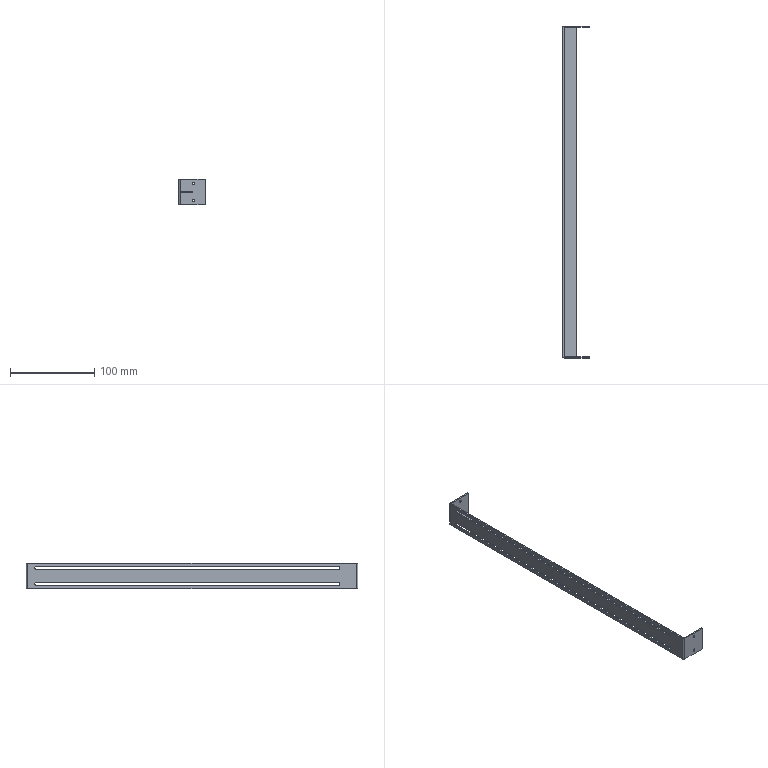Part | SolidWorks | features ICE 3, FlatPattern 1, SMBaseFlange 1, SheetMetal 1 | 1 solid | 46 faces | box 31.5 x 395 x 30 mm | volume 22778 mm3 | plane 26 | cylinder 20 | commonest cylinder face diameters 3.2 x14 1 x4 4 x2
STEP:
#1=CARTESIAN_POINT('',(0.,-174.5,26.2));
#2=VERTEX_POINT('',#1);
#3=CARTESIAN_POINT('',(0.,-176.1,24.6));
#4=VERTEX_POINT('',#3);
#5=CARTESIAN_POINT('',(0.,-174.5,24.6));
#6=DIRECTION('',(1.,0.,0.));
#7=DIRECTION('',(0.,1.,0.));
#8=AXIS2_PLACEMENT_3D('',#5,#6,#7);
#9=CIRCLE('',#8,1.6);
#10=EDGE_CURVE('',#2,#4,#9,.T.);
#11=ORIENTED_EDGE('',*,*,#10,.T.);
#12=CARTESIAN_POINT('',(-1.5,-176.1,24.6));
#13=VERTEX_POINT('',#12);
#14=CARTESIAN_POINT('',(30.,-176.1,24.6));
#15=DIRECTION('',(-1.,0.,0.));
#16=VECTOR('',#15,1000.);
#17=LINE('',#14,#16);
#18=EDGE_CURVE('',#4,#13,#17,.T.);
#19=ORIENTED_EDGE('',*,*,#18,.T.);
#20=CARTESIAN_POINT('',(-1.5,-174.5,26.2));
#21=VERTEX_POINT('',#20);
#22=CARTESIAN_POINT('',(-1.5,-174.5,24.6));
#23=DIRECTION('',(-1.,0.,0.));
#24=DIRECTION('',(0.,-1.,0.));
#25=AXIS2_PLACEMENT_3D('',#22,#23,#24);
#26=CIRCLE('',#25,1.6);
#27=EDGE_CURVE('',#13,#21,#26,.T.);
#28=ORIENTED_EDGE('',*,*,#27,.T.);
#29=CARTESIAN_POINT('',(30.,-174.5,26.2));
#30=DIRECTION('',(-1.,0.,0.));
#31=VECTOR('',#30,1000.);
#32=LINE('',#29,#31);
#33=EDGE_CURVE('',#2,#21,#32,.T.);
#34=ORIENTED_EDGE('',*,*,#33,.F.);
#35=EDGE_LOOP('',(#11,#19,#28,#34));
#36=FACE_OUTER_BOUND('',#35,.T.);
#37=CARTESIAN_POINT('',(30.,-174.5,24.6));
#38=DIRECTION('',(-1.,0.,0.));
#39=DIRECTION('',(0.,-1.,0.));
#40=AXIS2_PLACEMENT_3D('',#37,#38,#39);
#41=CYLINDRICAL_SURFACE('',#40,1.6);
#42=ADVANCED_FACE('',(#36),#41,.F.);
#43=CARTESIAN_POINT('',(0.,-174.5,7.2));
#44=VERTEX_POINT('',#43);
#45=CARTESIAN_POINT('',(0.,-176.1,5.6));
#46=VERTEX_POINT('',#45);
#47=CARTESIAN_POINT('',(0.,-174.5,5.6));
#48=DIRECTION('',(1.,0.,0.));
#49=DIRECTION('',(0.,1.,0.));
#50=AXIS2_PLACEMENT_3D('',#47,#48,#49);
#51=CIRCLE('',#50,1.6);
#52=EDGE_CURVE('',#44,#46,#51,.T.);
#53=ORIENTED_EDGE('',*,*,#52,.T.);
#54=CARTESIAN_POINT('',(-1.5,-176.1,5.6));
#55=VERTEX_POINT('',#54);
#56=CARTESIAN_POINT('',(30.,-176.1,5.6));
#57=DIRECTION('',(-1.,0.,0.));
#58=VECTOR('',#57,1000.);
#59=LINE('',#56,#58);
#60=EDGE_CURVE('',#46,#55,#59,.T.);
#61=ORIENTED_EDGE('',*,*,#60,.T.);
#62=CARTESIAN_POINT('',(-1.5,-174.5,7.2));
#63=VERTEX_POINT('',#62);
#64=CARTESIAN_POINT('',(-1.5,-174.5,5.6));
#65=DIRECTION('',(-1.,0.,0.));
#66=DIRECTION('',(0.,-1.,0.));
#67=AXIS2_PLACEMENT_3D('',#64,#65,#66);
#68=CIRCLE('',#67,1.6);
#69=EDGE_CURVE('',#55,#63,#68,.T.);
#70=ORIENTED_EDGE('',*,*,#69,.T.);
#71=CARTESIAN_POINT('',(30.,-174.5,7.2));
#72=DIRECTION('',(-1.,0.,0.));
#73=VECTOR('',#72,1000.);
#74=LINE('',#71,#73);
#75=EDGE_CURVE('',#44,#63,#74,.T.);
#76=ORIENTED_EDGE('',*,*,#75,.F.);
#77=EDGE_LOOP('',(#53,#61,#70,#76));
#78=FACE_OUTER_BOUND('',#77,.T.);
#79=CARTESIAN_POINT('',(30.,-174.5,5.6));
#80=DIRECTION('',(-1.,0.,0.));
#81=DIRECTION('',(0.,-1.,0.));
#82=AXIS2_PLACEMENT_3D('',#79,#80,#81);
#83=CYLINDRICAL_SURFACE('',#82,1.6);
#84=ADVANCED_FACE('',(#78),#83,.F.);
#85=CARTESIAN_POINT('',(16.,-196.,3.4));
#86=VERTEX_POINT('',#85);
#87=CARTESIAN_POINT('',(16.,-196.,6.6));
#88=VERTEX_POINT('',#87);
#89=CARTESIAN_POINT('',(16.,-196.,5.));
#90=DIRECTION('',(0.,1.,0.));
#91=DIRECTION('',(0.,0.,1.));
#92=AXIS2_PLACEMENT_3D('',#89,#90,#91);
#93=CIRCLE('',#92,1.6);
#94=EDGE_CURVE('',#86,#88,#93,.T.);
#95=ORIENTED_EDGE('',*,*,#94,.T.);
#96=CARTESIAN_POINT('',(16.,-197.5,6.6));
#97=VERTEX_POINT('',#96);
#98=CARTESIAN_POINT('',(16.,197.5,6.6));
#99=DIRECTION('',(0.,-1.,0.));
#100=VECTOR('',#99,1000.);
#101=LINE('',#98,#100);
#102=EDGE_CURVE('',#88,#97,#101,.T.);
#103=ORIENTED_EDGE('',*,*,#102,.T.);
#104=CARTESIAN_POINT('',(16.,-197.5,3.4));
#105=VERTEX_POINT('',#104);
#106=CARTESIAN_POINT('',(16.,-197.5,5.));
#107=DIRECTION('',(0.,-1.,0.));
#108=DIRECTION('',(0.,0.,-1.));
#109=AXIS2_PLACEMENT_3D('',#106,#107,#108);
#110=CIRCLE('',#109,1.6);
#111=EDGE_CURVE('',#97,#105,#110,.T.);
#112=ORIENTED_EDGE('',*,*,#111,.T.);
#113=CARTESIAN_POINT('',(16.,197.5,3.4));
#114=DIRECTION('',(0.,-1.,0.));
#115=VECTOR('',#114,1000.);
#116=LINE('',#113,#115);
#117=EDGE_CURVE('',#86,#105,#116,.T.);
#118=ORIENTED_EDGE('',*,*,#117,.F.);
#119=EDGE_LOOP('',(#95,#103,#112,#118));
#120=FACE_OUTER_BOUND('',#119,.T.);
#121=CARTESIAN_POINT('',(16.,197.5,5.));
#122=DIRECTION('',(0.,-1.,0.));
#123=DIRECTION('',(0.,0.,-1.));
#124=AXIS2_PLACEMENT_3D('',#121,#122,#123);
#125=CYLINDRICAL_SURFACE('',#124,1.6);
#126=ADVANCED_FACE('',(#120),#125,.F.);
#127=CARTESIAN_POINT('',(16.,197.5,6.6));
#128=VERTEX_POINT('',#127);
#129=CARTESIAN_POINT('',(16.,197.5,3.4));
#130=VERTEX_POINT('',#129);
#131=CARTESIAN_POINT('',(16.,197.5,5.));
#132=DIRECTION('',(0.,-1.,0.));
#133=DIRECTION('',(0.,0.,-1.));
#134=AXIS2_PLACEMENT_3D('',#131,#132,#133);
#135=CIRCLE('',#134,1.6);
#136=EDGE_CURVE('',#128,#130,#135,.T.);
#137=ORIENTED_EDGE('',*,*,#136,.F.);
#138=CARTESIAN_POINT('',(16.,196.,6.6));
#139=VERTEX_POINT('',#138);
#140=CARTESIAN_POINT('',(16.,197.5,6.6));
#141=DIRECTION('',(0.,-1.,0.));
#142=VECTOR('',#141,1000.);
#143=LINE('',#140,#142);
#144=EDGE_CURVE('',#128,#139,#143,.T.);
#145=ORIENTED_EDGE('',*,*,#144,.T.);
#146=CARTESIAN_POINT('',(16.,196.,3.4));
#147=VERTEX_POINT('',#146);
#148=CARTESIAN_POINT('',(16.,196.,5.));
#149=DIRECTION('',(0.,-1.,0.));
#150=DIRECTION('',(0.,0.,-1.));
#151=AXIS2_PLACEMENT_3D('',#148,#149,#150);
#152=CIRCLE('',#151,1.6);
#153=EDGE_CURVE('',#139,#147,#152,.T.);
#154=ORIENTED_EDGE('',*,*,#153,.T.);
#155=CARTESIAN_POINT('',(16.,197.5,3.4));
#156=DIRECTION('',(0.,-1.,0.));
#157=VECTOR('',#156,1000.);
#158=LINE('',#155,#157);
#159=EDGE_CURVE('',#130,#147,#158,.T.);
#160=ORIENTED_EDGE('',*,*,#159,.F.);
#161=EDGE_LOOP('',(#137,#145,#154,#160));
#162=FACE_OUTER_BOUND('',#161,.T.);
#163=CARTESIAN_POINT('',(16.,197.5,5.));
#164=DIRECTION('',(0.,-1.,0.));
#165=DIRECTION('',(0.,0.,-1.));
#166=AXIS2_PLACEMENT_3D('',#163,#164,#165);
#167=CYLINDRICAL_SURFACE('',#166,1.6);
#168=ADVANCED_FACE('',(#162),#167,.F.);
#169=CARTESIAN_POINT('',(16.,-196.,23.4));
#170=VERTEX_POINT('',#169);
#171=CARTESIAN_POINT('',(16.,-196.,26.6));
#172=VERTEX_POINT('',#171);
#173=CARTESIAN_POINT('',(16.,-196.,25.));
#174=DIRECTION('',(0.,1.,0.));
#175=DIRECTION('',(0.,0.,1.));
#176=AXIS2_PLACEMENT_3D('',#173,#174,#175);
#177=CIRCLE('',#176,1.6);
#178=EDGE_CURVE('',#170,#172,#177,.T.);
#179=ORIENTED_EDGE('',*,*,#178,.T.);
#180=CARTESIAN_POINT('',(16.,-197.5,26.6));
#181=VERTEX_POINT('',#180);
#182=CARTESIAN_POINT('',(16.,197.5,26.6));
#183=DIRECTION('',(0.,-1.,0.));
#184=VECTOR('',#183,1000.);
#185=LINE('',#182,#184);
#186=EDGE_CURVE('',#172,#181,#185,.T.);
#187=ORIENTED_EDGE('',*,*,#186,.T.);
#188=CARTESIAN_POINT('',(16.,-197.5,23.4));
#189=VERTEX_POINT('',#188);
#190=CARTESIAN_POINT('',(16.,-197.5,25.));
#191=DIRECTION('',(0.,-1.,0.));
#192=DIRECTION('',(0.,0.,-1.));
#193=AXIS2_PLACEMENT_3D('',#190,#191,#192);
#194=CIRCLE('',#193,1.6);
#195=EDGE_CURVE('',#181,#189,#194,.T.);
#196=ORIENTED_EDGE('',*,*,#195,.T.);
#197=CARTESIAN_POINT('',(16.,197.5,23.4));
#198=DIRECTION('',(0.,-1.,0.));
#199=VECTOR('',#198,1000.);
#200=LINE('',#197,#199);
#201=EDGE_CURVE('',#170,#189,#200,.T.);
#202=ORIENTED_EDGE('',*,*,#201,.F.);
#203=EDGE_LOOP('',(#179,#187,#196,#202));
#204=FACE_OUTER_BOUND('',#203,.T.);
#205=CARTESIAN_POINT('',(16.,197.5,25.));
#206=DIRECTION('',(0.,-1.,0.));
#207=DIRECTION('',(0.,0.,-1.));
#208=AXIS2_PLACEMENT_3D('',#205,#206,#207);
#209=CYLINDRICAL_SURFACE('',#208,1.6);
#210=ADVANCED_FACE('',(#204),#209,.F.);
#211=CARTESIAN_POINT('',(16.,197.5,26.6));
#212=VERTEX_POINT('',#211);
#213=CARTESIAN_POINT('',(16.,197.5,23.4));
#214=VERTEX_POINT('',#213);
#215=CARTESIAN_POINT('',(16.,197.5,25.));
#216=DIRECTION('',(0.,-1.,0.));
#217=DIRECTION('',(0.,0.,-1.));
#218=AXIS2_PLACEMENT_3D('',#215,#216,#217);
#219=CIRCLE('',#218,1.6);
#220=EDGE_CURVE('',#212,#214,#219,.T.);
#221=ORIENTED_EDGE('',*,*,#220,.F.);
#222=CARTESIAN_POINT('',(16.,196.,26.6));
#223=VERTEX_POINT('',#222);
#224=CARTESIAN_POINT('',(16.,197.5,26.6));
#225=DIRECTION('',(0.,-1.,0.));
#226=VECTOR('',#225,1000.);
#227=LINE('',#224,#226);
#228=EDGE_CURVE('',#212,#223,#227,.T.);
#229=ORIENTED_EDGE('',*,*,#228,.T.);
#230=CARTESIAN_POINT('',(16.,196.,23.4));
#231=VERTEX_POINT('',#230);
#232=CARTESIAN_POINT('',(16.,196.,25.));
#233=DIRECTION('',(0.,-1.,0.));
#234=DIRECTION('',(0.,0.,-1.));
#235=AXIS2_PLACEMENT_3D('',#232,#233,#234);
#236=CIRCLE('',#235,1.6);
#237=EDGE_CURVE('',#223,#231,#236,.T.);
#238=ORIENTED_EDGE('',*,*,#237,.T.);
#239=CARTESIAN_POINT('',(16.,197.5,23.4));
#240=DIRECTION('',(0.,-1.,0.));
#241=VECTOR('',#240,1000.);
#242=LINE('',#239,#241);
#243=EDGE_CURVE('',#214,#231,#242,.T.);
#244=ORIENTED_EDGE('',*,*,#243,.F.);
#245=EDGE_LOOP('',(#221,#229,#238,#244));
#246=FACE_OUTER_BOUND('',#245,.T.);
#247=CARTESIAN_POINT('',(16.,197.5,25.));
#248=DIRECTION('',(0.,-1.,0.));
#249=DIRECTION('',(0.,0.,-1.));
#250=AXIS2_PLACEMENT_3D('',#247,#248,#249);
#251=CYLINDRICAL_SURFACE('',#250,1.6);
#252=ADVANCED_FACE('',(#246),#251,.F.);
#253=ORIENTED_EDGE('',*,*,#178,.F.);
#254=CARTESIAN_POINT('',(16.,-196.,25.));
#255=DIRECTION('',(0.,1.,0.));
#256=DIRECTION('',(0.,0.,1.));
#257=AXIS2_PLACEMENT_3D('',#254,#255,#256);
#258=CIRCLE('',#257,1.6);
#259=EDGE_CURVE('',#172,#170,#258,.T.);
#260=ORIENTED_EDGE('',*,*,#259,.F.);
#261=EDGE_LOOP('',(#253,#260));
#262=FACE_BOUND('',#261,.T.);
#263=ORIENTED_EDGE('',*,*,#94,.F.);
#264=CARTESIAN_POINT('',(16.,-196.,5.));
#265=DIRECTION('',(0.,1.,0.));
#266=DIRECTION('',(0.,0.,1.));
#267=AXIS2_PLACEMENT_3D('',#264,#265,#266);
#268=CIRCLE('',#267,1.6);
#269=EDGE_CURVE('',#88,#86,#268,.T.);
#270=ORIENTED_EDGE('',*,*,#269,.F.);
#271=EDGE_LOOP('',(#263,#270));
#272=FACE_BOUND('',#271,.T.);
#273=CARTESIAN_POINT('',(15.,-196.,15.5));
#274=VERTEX_POINT('',#273);
#275=CARTESIAN_POINT('',(15.,-196.,14.5));
#276=VERTEX_POINT('',#275);
#277=CARTESIAN_POINT('',(15.,-196.,15.5));
#278=DIRECTION('',(0.,0.,-1.));
#279=VECTOR('',#278,1000.);
#280=LINE('',#277,#279);
#281=EDGE_CURVE('',#274,#276,#280,.T.);
#282=ORIENTED_EDGE('',*,*,#281,.F.);
#283=CARTESIAN_POINT('',(0.5,-196.,15.5));
#284=VERTEX_POINT('',#283);
#285=CARTESIAN_POINT('',(15.,-196.,15.5));
#286=DIRECTION('',(-1.,0.,0.));
#287=VECTOR('',#286,1000.);
#288=LINE('',#285,#287);
#289=EDGE_CURVE('',#274,#284,#288,.T.);
#290=ORIENTED_EDGE('',*,*,#289,.T.);
#291=CARTESIAN_POINT('',(0.5,-196.,30.));
#292=VERTEX_POINT('',#291);
#293=CARTESIAN_POINT('',(0.5,-196.,30.));
#294=DIRECTION('',(0.,0.,-1.));
#295=VECTOR('',#294,1000.);
#296=LINE('',#293,#295);
#297=EDGE_CURVE('',#292,#284,#296,.T.);
#298=ORIENTED_EDGE('',*,*,#297,.F.);
#299=CARTESIAN_POINT('',(30.,-196.,30.));
#300=VERTEX_POINT('',#299);
#301=CARTESIAN_POINT('',(0.,-196.,30.));
#302=DIRECTION('',(1.,0.,0.));
#303=VECTOR('',#302,1000.);
#304=LINE('',#301,#303);
#305=EDGE_CURVE('',#292,#300,#304,.T.);
#306=ORIENTED_EDGE('',*,*,#305,.T.);
#307=CARTESIAN_POINT('',(30.,-196.,0.));
#308=VERTEX_POINT('',#307);
#309=CARTESIAN_POINT('',(30.,-196.,30.));
#310=DIRECTION('',(0.,0.,-1.));
#311=VECTOR('',#310,1000.);
#312=LINE('',#309,#311);
#313=EDGE_CURVE('',#300,#308,#312,.T.);
#314=ORIENTED_EDGE('',*,*,#313,.T.);
#315=CARTESIAN_POINT('',(0.5,-196.,0.));
#316=VERTEX_POINT('',#315);
#317=CARTESIAN_POINT('',(0.,-196.,0.));
#318=DIRECTION('',(1.,0.,0.));
#319=VECTOR('',#318,1000.);
#320=LINE('',#317,#319);
#321=EDGE_CURVE('',#316,#308,#320,.T.);
#322=ORIENTED_EDGE('',*,*,#321,.F.);
#323=CARTESIAN_POINT('',(0.5,-196.,14.5));
#324=VERTEX_POINT('',#323);
#325=CARTESIAN_POINT('',(0.5,-196.,30.));
#326=DIRECTION('',(0.,0.,-1.));
#327=VECTOR('',#326,1000.);
#328=LINE('',#325,#327);
#329=EDGE_CURVE('',#324,#316,#328,.T.);
#330=ORIENTED_EDGE('',*,*,#329,.F.);
#331=CARTESIAN_POINT('',(15.,-196.,14.5));
#332=DIRECTION('',(-1.,0.,0.));
#333=VECTOR('',#332,1000.);
#334=LINE('',#331,#333);
#335=EDGE_CURVE('',#276,#324,#334,.T.);
#336=ORIENTED_EDGE('',*,*,#335,.F.);
#337=EDGE_LOOP('',(#282,#290,#298,#306,#314,#322,#330,#336));
#338=FACE_OUTER_BOUND('',#337,.T.);
#339=CARTESIAN_POINT('',(0.,-196.,30.));
#340=DIRECTION('',(0.,1.,0.));
#341=DIRECTION('',(0.,0.,1.));
#342=AXIS2_PLACEMENT_3D('',#339,#340,#341);
#343=PLANE('',#342);
#344=ADVANCED_FACE('',(#262,#272,#338),#343,.T.);
#345=ORIENTED_EDGE('',*,*,#297,.T.);
#346=CARTESIAN_POINT('',(0.,-195.5,15.5));
#347=VERTEX_POINT('',#346);
#348=CARTESIAN_POINT('',(0.5,-195.5,15.5));
#349=DIRECTION('',(0.,0.,-1.));
#350=DIRECTION('',(0.,1.,0.));
#351=AXIS2_PLACEMENT_3D('',#348,#349,#350);
#352=CIRCLE('',#351,0.5);
#353=EDGE_CURVE('',#284,#347,#352,.T.);
#354=ORIENTED_EDGE('',*,*,#353,.T.);
#355=CARTESIAN_POINT('',(0.,-195.5,30.));
#356=VERTEX_POINT('',#355);
#357=CARTESIAN_POINT('',(0.,-195.5,30.));
#358=DIRECTION('',(0.,0.,-1.));
#359=VECTOR('',#358,1000.);
#360=LINE('',#357,#359);
#361=EDGE_CURVE('',#356,#347,#360,.T.);
#362=ORIENTED_EDGE('',*,*,#361,.F.);
#363=CARTESIAN_POINT('',(0.5,-195.5,30.));
#364=DIRECTION('',(0.,0.,1.));
#365=DIRECTION('',(-1.,0.,0.));
#366=AXIS2_PLACEMENT_3D('',#363,#364,#365);
#367=CIRCLE('',#366,0.5);
#368=EDGE_CURVE('',#356,#292,#367,.T.);
#369=ORIENTED_EDGE('',*,*,#368,.T.);
#370=EDGE_LOOP('',(#345,#354,#362,#369));
#371=FACE_OUTER_BOUND('',#370,.T.);
#372=CARTESIAN_POINT('',(0.5,-195.5,30.));
#373=DIRECTION('',(0.,0.,-1.));
#374=DIRECTION('',(-1.,0.,0.));
#375=AXIS2_PLACEMENT_3D('',#372,#373,#374);
#376=CYLINDRICAL_SURFACE('',#375,0.5);
#377=ADVANCED_FACE('',(#371),#376,.F.);
#378=CARTESIAN_POINT('',(0.,-195.5,14.5));
#379=VERTEX_POINT('',#378);
#380=CARTESIAN_POINT('',(0.,-195.5,0.));
#381=VERTEX_POINT('',#380);
#382=CARTESIAN_POINT('',(0.,-195.5,30.));
#383=DIRECTION('',(0.,0.,-1.));
#384=VECTOR('',#383,1000.);
#385=LINE('',#382,#384);
#386=EDGE_CURVE('',#379,#381,#385,.T.);
#387=ORIENTED_EDGE('',*,*,#386,.F.);
#388=CARTESIAN_POINT('',(0.5,-195.5,14.5));
#389=DIRECTION('',(0.,0.,1.));
#390=DIRECTION('',(0.,-1.,0.));
#391=AXIS2_PLACEMENT_3D('',#388,#389,#390);
#392=CIRCLE('',#391,0.5);
#393=EDGE_CURVE('',#379,#324,#392,.T.);
#394=ORIENTED_EDGE('',*,*,#393,.T.);
#395=ORIENTED_EDGE('',*,*,#329,.T.);
#396=CARTESIAN_POINT('',(0.5,-195.5,0.));
#397=DIRECTION('',(0.,0.,1.));
#398=DIRECTION('',(-1.,0.,0.));
#399=AXIS2_PLACEMENT_3D('',#396,#397,#398);
#400=CIRCLE('',#399,0.5);
#401=EDGE_CURVE('',#381,#316,#400,.T.);
#402=ORIENTED_EDGE('',*,*,#401,.F.);
#403=EDGE_LOOP('',(#387,#394,#395,#402));
#404=FACE_OUTER_BOUND('',#403,.T.);
#405=CARTESIAN_POINT('',(0.5,-195.5,30.));
#406=DIRECTION('',(0.,0.,-1.));
#407=DIRECTION('',(-1.,0.,0.));
#408=AXIS2_PLACEMENT_3D('',#405,#406,#407);
#409=CYLINDRICAL_SURFACE('',#408,0.5);
#410=ADVANCED_FACE('',(#404),#409,.F.);
#411=CARTESIAN_POINT('',(0.,185.5,23.));
#412=VERTEX_POINT('',#411);
#413=CARTESIAN_POINT('',(0.,185.5,26.2));
#414=VERTEX_POINT('',#413);
#415=CARTESIAN_POINT('',(0.,185.5,24.6));
#416=DIRECTION('',(1.,0.,0.));
#417=DIRECTION('',(0.,1.,0.));
#418=AXIS2_PLACEMENT_3D('',#415,#416,#417);
#419=CIRCLE('',#418,1.6);
#420=EDGE_CURVE('',#412,#414,#419,.T.);
#421=ORIENTED_EDGE('',*,*,#420,.F.);
#422=CARTESIAN_POINT('',(0.,-174.5,23.));
#423=VERTEX_POINT('',#422);
#424=CARTESIAN_POINT('',(0.,196.,23.));
#425=DIRECTION('',(0.,1.,0.));
#426=VECTOR('',#425,1000.);
#427=LINE('',#424,#426);
#428=EDGE_CURVE('',#423,#412,#427,.T.);
#429=ORIENTED_EDGE('',*,*,#428,.F.);
#430=CARTESIAN_POINT('',(0.,-174.5,24.6));
#431=DIRECTION('',(1.,0.,0.));
#432=DIRECTION('',(0.,1.,0.));
#433=AXIS2_PLACEMENT_3D('',#430,#431,#432);
#434=CIRCLE('',#433,1.6);
#435=EDGE_CURVE('',#4,#423,#434,.T.);
#436=ORIENTED_EDGE('',*,*,#435,.F.);
#437=ORIENTED_EDGE('',*,*,#10,.F.);
#438=CARTESIAN_POINT('',(0.,196.,26.2));
#439=DIRECTION('',(0.,-1.,0.));
#440=VECTOR('',#439,1000.);
#441=LINE('',#438,#440);
#442=EDGE_CURVE('',#414,#2,#441,.T.);
#443=ORIENTED_EDGE('',*,*,#442,.F.);
#444=EDGE_LOOP('',(#421,#429,#436,#437,#443));
#445=FACE_BOUND('',#444,.T.);
#446=ORIENTED_EDGE('',*,*,#361,.T.);
#447=CARTESIAN_POINT('',(0.,195.5,15.5));
#448=VERTEX_POINT('',#447);
#449=CARTESIAN_POINT('',(0.,196.,15.5));
#450=DIRECTION('',(0.,-1.,0.));
#451=VECTOR('',#450,1000.);
#452=LINE('',#449,#451);
#453=EDGE_CURVE('',#448,#347,#452,.T.);
#454=ORIENTED_EDGE('',*,*,#453,.F.);
#455=CARTESIAN_POINT('',(0.,195.5,30.));
#456=VERTEX_POINT('',#455);
#457=CARTESIAN_POINT('',(0.,195.5,30.));
#458=DIRECTION('',(0.,0.,-1.));
#459=VECTOR('',#458,1000.);
#460=LINE('',#457,#459);
#461=EDGE_CURVE('',#456,#448,#460,.T.);
#462=ORIENTED_EDGE('',*,*,#461,.F.);
#463=CARTESIAN_POINT('',(0.,196.,30.));
#464=DIRECTION('',(0.,-1.,0.));
#465=VECTOR('',#464,1000.);
#466=LINE('',#463,#465);
#467=EDGE_CURVE('',#456,#356,#466,.T.);
#468=ORIENTED_EDGE('',*,*,#467,.T.);
#469=EDGE_LOOP('',(#446,#454,#462,#468));
#470=FACE_OUTER_BOUND('',#469,.T.);
#471=CARTESIAN_POINT('',(0.,196.,30.));
#472=DIRECTION('',(1.,0.,0.));
#473=DIRECTION('',(0.,1.,0.));
#474=AXIS2_PLACEMENT_3D('',#471,#472,#473);
#475=PLANE('',#474);
#476=ADVANCED_FACE('',(#445,#470),#475,.T.);
#477=CARTESIAN_POINT('',(0.,185.5,4.));
#478=VERTEX_POINT('',#477);
#479=CARTESIAN_POINT('',(0.,185.5,7.2));
#480=VERTEX_POINT('',#479);
#481=CARTESIAN_POINT('',(0.,185.5,5.6));
#482=DIRECTION('',(1.,0.,0.));
#483=DIRECTION('',(0.,1.,0.));
#484=AXIS2_PLACEMENT_3D('',#481,#482,#483);
#485=CIRCLE('',#484,1.6);
#486=EDGE_CURVE('',#478,#480,#485,.T.);
#487=ORIENTED_EDGE('',*,*,#486,.F.);
#488=CARTESIAN_POINT('',(0.,-174.5,4.));
#489=VERTEX_POINT('',#488);
#490=CARTESIAN_POINT('',(0.,196.,4.));
#491=DIRECTION('',(0.,1.,0.));
#492=VECTOR('',#491,1000.);
#493=LINE('',#490,#492);
#494=EDGE_CURVE('',#489,#478,#493,.T.);
#495=ORIENTED_EDGE('',*,*,#494,.F.);
#496=CARTESIAN_POINT('',(0.,-174.5,5.6));
#497=DIRECTION('',(1.,0.,0.));
#498=DIRECTION('',(0.,1.,0.));
#499=AXIS2_PLACEMENT_3D('',#496,#497,#498);
#500=CIRCLE('',#499,1.6);
#501=EDGE_CURVE('',#46,#489,#500,.T.);
#502=ORIENTED_EDGE('',*,*,#501,.F.);
#503=ORIENTED_EDGE('',*,*,#52,.F.);
#504=CARTESIAN_POINT('',(0.,196.,7.2));
#505=DIRECTION('',(0.,-1.,0.));
#506=VECTOR('',#505,1000.);
#507=LINE('',#504,#506);
#508=EDGE_CURVE('',#480,#44,#507,.T.);
#509=ORIENTED_EDGE('',*,*,#508,.F.);
#510=EDGE_LOOP('',(#487,#495,#502,#503,#509));
#511=FACE_BOUND('',#510,.T.);
#512=CARTESIAN_POINT('',(0.,195.5,14.5));
#513=VERTEX_POINT('',#512);
#514=CARTESIAN_POINT('',(0.,195.5,0.));
#515=VERTEX_POINT('',#514);
#516=CARTESIAN_POINT('',(0.,195.5,30.));
#517=DIRECTION('',(0.,0.,-1.));
#518=VECTOR('',#517,1000.);
#519=LINE('',#516,#518);
#520=EDGE_CURVE('',#513,#515,#519,.T.);
#521=ORIENTED_EDGE('',*,*,#520,.F.);
#522=CARTESIAN_POINT('',(0.,196.,14.5));
#523=DIRECTION('',(0.,1.,0.));
#524=VECTOR('',#523,1000.);
#525=LINE('',#522,#524);
#526=EDGE_CURVE('',#379,#513,#525,.T.);
#527=ORIENTED_EDGE('',*,*,#526,.F.);
#528=ORIENTED_EDGE('',*,*,#386,.T.);
#529=CARTESIAN_POINT('',(0.,196.,0.));
#530=DIRECTION('',(0.,-1.,0.));
#531=VECTOR('',#530,1000.);
#532=LINE('',#529,#531);
#533=EDGE_CURVE('',#515,#381,#532,.T.);
#534=ORIENTED_EDGE('',*,*,#533,.F.);
#535=EDGE_LOOP('',(#521,#527,#528,#534));
#536=FACE_OUTER_BOUND('',#535,.T.);
#537=CARTESIAN_POINT('',(0.,196.,30.));
#538=DIRECTION('',(1.,0.,0.));
#539=DIRECTION('',(0.,1.,0.));
#540=AXIS2_PLACEMENT_3D('',#537,#538,#539);
#541=PLANE('',#540);
#542=ADVANCED_FACE('',(#511,#536),#541,.T.);
#543=ORIENTED_EDGE('',*,*,#461,.T.);
#544=CARTESIAN_POINT('',(0.5,196.,15.5));
#545=VERTEX_POINT('',#544);
#546=CARTESIAN_POINT('',(0.5,195.5,15.5));
#547=DIRECTION('',(0.,0.,-1.));
#548=DIRECTION('',(0.,1.,0.));
#549=AXIS2_PLACEMENT_3D('',#546,#547,#548);
#550=CIRCLE('',#549,0.5);
#551=EDGE_CURVE('',#448,#545,#550,.T.);
#552=ORIENTED_EDGE('',*,*,#551,.T.);
#553=CARTESIAN_POINT('',(0.5,196.,30.));
#554=VERTEX_POINT('',#553);
#555=CARTESIAN_POINT('',(0.5,196.,30.));
#556=DIRECTION('',(0.,0.,-1.));
#557=VECTOR('',#556,1000.);
#558=LINE('',#555,#557);
#559=EDGE_CURVE('',#554,#545,#558,.T.);
#560=ORIENTED_EDGE('',*,*,#559,.F.);
#561=CARTESIAN_POINT('',(0.5,195.5,30.));
#562=DIRECTION('',(0.,0.,1.));
#563=DIRECTION('',(-1.,0.,0.));
#564=AXIS2_PLACEMENT_3D('',#561,#562,#563);
#565=CIRCLE('',#564,0.5);
#566=EDGE_CURVE('',#554,#456,#565,.T.);
#567=ORIENTED_EDGE('',*,*,#566,.T.);
#568=EDGE_LOOP('',(#543,#552,#560,#567));
#569=FACE_OUTER_BOUND('',#568,.T.);
#570=CARTESIAN_POINT('',(0.5,195.5,30.));
#571=DIRECTION('',(0.,0.,-1.));
#572=DIRECTION('',(-1.,0.,0.));
#573=AXIS2_PLACEMENT_3D('',#570,#571,#572);
#574=CYLINDRICAL_SURFACE('',#573,0.5);
#575=ADVANCED_FACE('',(#569),#574,.F.);
#576=CARTESIAN_POINT('',(0.5,196.,14.5));
#577=VERTEX_POINT('',#576);
#578=CARTESIAN_POINT('',(0.5,196.,0.));
#579=VERTEX_POINT('',#578);
#580=CARTESIAN_POINT('',(0.5,196.,30.));
#581=DIRECTION('',(0.,0.,-1.));
#582=VECTOR('',#581,1000.);
#583=LINE('',#580,#582);
#584=EDGE_CURVE('',#577,#579,#583,.T.);
#585=ORIENTED_EDGE('',*,*,#584,.F.);
#586=CARTESIAN_POINT('',(0.5,195.5,14.5));
#587=DIRECTION('',(0.,0.,1.));
#588=DIRECTION('',(0.,-1.,0.));
#589=AXIS2_PLACEMENT_3D('',#586,#587,#588);
#590=CIRCLE('',#589,0.5);
#591=EDGE_CURVE('',#577,#513,#590,.T.);
#592=ORIENTED_EDGE('',*,*,#591,.T.);
#593=ORIENTED_EDGE('',*,*,#520,.T.);
#594=CARTESIAN_POINT('',(0.5,195.5,0.));
#595=DIRECTION('',(0.,0.,1.));
#596=DIRECTION('',(-1.,0.,0.));
#597=AXIS2_PLACEMENT_3D('',#594,#595,#596);
#598=CIRCLE('',#597,0.5);
#599=EDGE_CURVE('',#579,#515,#598,.T.);
#600=ORIENTED_EDGE('',*,*,#599,.F.);
#601=EDGE_LOOP('',(#585,#592,#593,#600));
#602=FACE_OUTER_BOUND('',#601,.T.);
#603=CARTESIAN_POINT('',(0.5,195.5,30.));
#604=DIRECTION('',(0.,0.,-1.));
#605=DIRECTION('',(-1.,0.,0.));
#606=AXIS2_PLACEMENT_3D('',#603,#604,#605);
#607=CYLINDRICAL_SURFACE('',#606,0.5);
#608=ADVANCED_FACE('',(#602),#607,.F.);
#609=CARTESIAN_POINT('',(16.,196.,25.));
#610=DIRECTION('',(0.,-1.,0.));
#611=DIRECTION('',(0.,0.,-1.));
#612=AXIS2_PLACEMENT_3D('',#609,#610,#611);
#613=CIRCLE('',#612,1.6);
#614=EDGE_CURVE('',#231,#223,#613,.T.);
#615=ORIENTED_EDGE('',*,*,#614,.F.);
#616=ORIENTED_EDGE('',*,*,#237,.F.);
#617=EDGE_LOOP('',(#615,#616));
#618=FACE_BOUND('',#617,.T.);
#619=CARTESIAN_POINT('',(16.,196.,5.));
#620=DIRECTION('',(0.,-1.,0.));
#621=DIRECTION('',(0.,0.,-1.));
#622=AXIS2_PLACEMENT_3D('',#619,#620,#621);
#623=CIRCLE('',#622,1.6);
#624=EDGE_CURVE('',#147,#139,#623,.T.);
#625=ORIENTED_EDGE('',*,*,#624,.F.);
#626=ORIENTED_EDGE('',*,*,#153,.F.);
#627=EDGE_LOOP('',(#625,#626));
#628=FACE_BOUND('',#627,.T.);
#629=ORIENTED_EDGE('',*,*,#559,.T.);
#630=CARTESIAN_POINT('',(15.,196.,15.5));
#631=VERTEX_POINT('',#630);
#632=CARTESIAN_POINT('',(15.,196.,15.5));
#633=DIRECTION('',(-1.,0.,0.));
#634=VECTOR('',#633,1000.);
#635=LINE('',#632,#634);
#636=EDGE_CURVE('',#631,#545,#635,.T.);
#637=ORIENTED_EDGE('',*,*,#636,.F.);
#638=CARTESIAN_POINT('',(15.,196.,14.5));
#639=VERTEX_POINT('',#638);
#640=CARTESIAN_POINT('',(15.,196.,15.5));
#641=DIRECTION('',(0.,0.,1.));
#642=VECTOR('',#641,1000.);
#643=LINE('',#640,#642);
#644=EDGE_CURVE('',#639,#631,#643,.T.);
#645=ORIENTED_EDGE('',*,*,#644,.F.);
#646=CARTESIAN_POINT('',(15.,196.,14.5));
#647=DIRECTION('',(-1.,0.,0.));
#648=VECTOR('',#647,1000.);
#649=LINE('',#646,#648);
#650=EDGE_CURVE('',#639,#577,#649,.T.);
#651=ORIENTED_EDGE('',*,*,#650,.T.);
#652=ORIENTED_EDGE('',*,*,#584,.T.);
#653=CARTESIAN_POINT('',(30.,196.,0.));
#654=VERTEX_POINT('',#653);
#655=CARTESIAN_POINT('',(0.,196.,0.));
#656=DIRECTION('',(-1.,0.,0.));
#657=VECTOR('',#656,1000.);
#658=LINE('',#655,#657);
#659=EDGE_CURVE('',#654,#579,#658,.T.);
#660=ORIENTED_EDGE('',*,*,#659,.F.);
#661=CARTESIAN_POINT('',(30.,196.,30.));
#662=VERTEX_POINT('',#661);
#663=CARTESIAN_POINT('',(30.,196.,30.));
#664=DIRECTION('',(0.,0.,-1.));
#665=VECTOR('',#664,1000.);
#666=LINE('',#663,#665);
#667=EDGE_CURVE('',#662,#654,#666,.T.);
#668=ORIENTED_EDGE('',*,*,#667,.F.);
#669=CARTESIAN_POINT('',(0.,196.,30.));
#670=DIRECTION('',(-1.,0.,0.));
#671=VECTOR('',#670,1000.);
#672=LINE('',#669,#671);
#673=EDGE_CURVE('',#662,#554,#672,.T.);
#674=ORIENTED_EDGE('',*,*,#673,.T.);
#675=EDGE_LOOP('',(#629,#637,#645,#651,#652,#660,#668,#674));
#676=FACE_OUTER_BOUND('',#675,.T.);
#677=CARTESIAN_POINT('',(0.,196.,30.));
#678=DIRECTION('',(0.,-1.,0.));
#679=DIRECTION('',(0.,0.,-1.));
#680=AXIS2_PLACEMENT_3D('',#677,#678,#679);
#681=PLANE('',#680);
#682=ADVANCED_FACE('',(#618,#628,#676),#681,.T.);
#683=CARTESIAN_POINT('',(-1.5,195.5,30.));
#684=VERTEX_POINT('',#683);
#685=CARTESIAN_POINT('',(0.,195.5,30.));
#686=DIRECTION('',(-1.,0.,0.));
#687=VECTOR('',#686,1000.);
#688=LINE('',#685,#687);
#689=EDGE_CURVE('',#456,#684,#688,.T.);
#690=ORIENTED_EDGE('',*,*,#689,.F.);
#691=ORIENTED_EDGE('',*,*,#566,.F.);
#692=CARTESIAN_POINT('',(0.5,197.5,30.));
#693=VERTEX_POINT('',#692);
#694=CARTESIAN_POINT('',(0.5,197.5,30.));
#695=DIRECTION('',(0.,-1.,0.));
#696=VECTOR('',#695,1000.);
#697=LINE('',#694,#696);
#698=EDGE_CURVE('',#693,#554,#697,.T.);
#699=ORIENTED_EDGE('',*,*,#698,.F.);
#700=CARTESIAN_POINT('',(0.5,195.5,30.));
#701=DIRECTION('',(0.,0.,1.));
#702=DIRECTION('',(1.,0.,0.));
#703=AXIS2_PLACEMENT_3D('',#700,#701,#702);
#704=CIRCLE('',#703,2.);
#705=EDGE_CURVE('',#693,#684,#704,.T.);
#706=ORIENTED_EDGE('',*,*,#705,.T.);
#707=EDGE_LOOP('',(#690,#691,#699,#706));
#708=FACE_OUTER_BOUND('',#707,.T.);
#709=CARTESIAN_POINT('',(0.,195.5,30.));
#710=DIRECTION('',(0.,0.,1.));
#711=DIRECTION('',(1.,0.,0.));
#712=AXIS2_PLACEMENT_3D('',#709,#710,#711);
#713=PLANE('',#712);
#714=ADVANCED_FACE('',(#708),#713,.T.);
#715=ORIENTED_EDGE('',*,*,#467,.F.);
#716=ORIENTED_EDGE('',*,*,#689,.T.);
#717=CARTESIAN_POINT('',(-1.5,-195.5,30.));
#718=VERTEX_POINT('',#717);
#719=CARTESIAN_POINT('',(-1.5,196.,30.));
#720=DIRECTION('',(0.,-1.,0.));
#721=VECTOR('',#720,1000.);
#722=LINE('',#719,#721);
#723=EDGE_CURVE('',#684,#718,#722,.T.);
#724=ORIENTED_EDGE('',*,*,#723,.T.);
#725=CARTESIAN_POINT('',(-1.5,-195.5,30.));
#726=DIRECTION('',(1.,0.,0.));
#727=VECTOR('',#726,1000.);
#728=LINE('',#725,#727);
#729=EDGE_CURVE('',#718,#356,#728,.T.);
#730=ORIENTED_EDGE('',*,*,#729,.T.);
#731=EDGE_LOOP('',(#715,#716,#724,#730));
#732=FACE_OUTER_BOUND('',#731,.T.);
#733=CARTESIAN_POINT('',(0.5,197.5,30.));
#734=DIRECTION('',(0.,0.,1.));
#735=DIRECTION('',(1.,0.,0.));
#736=AXIS2_PLACEMENT_3D('',#733,#734,#735);
#737=PLANE('',#736);
#738=ADVANCED_FACE('',(#732),#737,.T.);
#739=CARTESIAN_POINT('',(0.5,197.5,0.));
#740=VERTEX_POINT('',#739);
#741=CARTESIAN_POINT('',(0.5,196.,0.));
#742=DIRECTION('',(0.,1.,0.));
#743=VECTOR('',#742,1000.);
#744=LINE('',#741,#743);
#745=EDGE_CURVE('',#579,#740,#744,.T.);
#746=ORIENTED_EDGE('',*,*,#745,.F.);
#747=ORIENTED_EDGE('',*,*,#599,.T.);
#748=CARTESIAN_POINT('',(-1.5,195.5,0.));
#749=VERTEX_POINT('',#748);
#750=CARTESIAN_POINT('',(-1.5,195.5,0.));
#751=DIRECTION('',(1.,0.,0.));
#752=VECTOR('',#751,1000.);
#753=LINE('',#750,#752);
#754=EDGE_CURVE('',#749,#515,#753,.T.);
#755=ORIENTED_EDGE('',*,*,#754,.F.);
#756=CARTESIAN_POINT('',(0.5,195.5,0.));
#757=DIRECTION('',(0.,0.,1.));
#758=DIRECTION('',(1.,0.,0.));
#759=AXIS2_PLACEMENT_3D('',#756,#757,#758);
#760=CIRCLE('',#759,2.);
#761=EDGE_CURVE('',#740,#749,#760,.T.);
#762=ORIENTED_EDGE('',*,*,#761,.F.);
#763=EDGE_LOOP('',(#746,#747,#755,#762));
#764=FACE_OUTER_BOUND('',#763,.T.);
#765=CARTESIAN_POINT('',(0.5,196.,0.));
#766=DIRECTION('',(0.,0.,-1.));
#767=DIRECTION('',(-1.,0.,0.));
#768=AXIS2_PLACEMENT_3D('',#765,#766,#767);
#769=PLANE('',#768);
#770=ADVANCED_FACE('',(#764),#769,.T.);
#771=ORIENTED_EDGE('',*,*,#659,.T.);
#772=ORIENTED_EDGE('',*,*,#745,.T.);
#773=CARTESIAN_POINT('',(30.,197.5,0.));
#774=VERTEX_POINT('',#773);
#775=CARTESIAN_POINT('',(0.,197.5,0.));
#776=DIRECTION('',(-1.,0.,0.));
#777=VECTOR('',#776,1000.);
#778=LINE('',#775,#777);
#779=EDGE_CURVE('',#774,#740,#778,.T.);
#780=ORIENTED_EDGE('',*,*,#779,.F.);
#781=CARTESIAN_POINT('',(30.,197.5,0.));
#782=DIRECTION('',(0.,-1.,0.));
#783=VECTOR('',#782,1000.);
#784=LINE('',#781,#783);
#785=EDGE_CURVE('',#774,#654,#784,.T.);
#786=ORIENTED_EDGE('',*,*,#785,.T.);
#787=EDGE_LOOP('',(#771,#772,#780,#786));
#788=FACE_OUTER_BOUND('',#787,.T.);
#789=CARTESIAN_POINT('',(-1.5,195.5,0.));
#790=DIRECTION('',(0.,0.,-1.));
#791=DIRECTION('',(-1.,0.,0.));
#792=AXIS2_PLACEMENT_3D('',#789,#790,#791);
#793=PLANE('',#792);
#794=ADVANCED_FACE('',(#788),#793,.T.);
#795=CARTESIAN_POINT('',(0.5,-197.5,30.));
#796=VERTEX_POINT('',#795);
#797=CARTESIAN_POINT('',(0.5,-196.,30.));
#798=DIRECTION('',(0.,-1.,0.));
#799=VECTOR('',#798,1000.);
#800=LINE('',#797,#799);
#801=EDGE_CURVE('',#292,#796,#800,.T.);
#802=ORIENTED_EDGE('',*,*,#801,.F.);
#803=ORIENTED_EDGE('',*,*,#368,.F.);
#804=ORIENTED_EDGE('',*,*,#729,.F.);
#805=CARTESIAN_POINT('',(0.5,-195.5,30.));
#806=DIRECTION('',(0.,0.,1.));
#807=DIRECTION('',(1.,0.,0.));
#808=AXIS2_PLACEMENT_3D('',#805,#806,#807);
#809=CIRCLE('',#808,2.);
#810=EDGE_CURVE('',#718,#796,#809,.T.);
#811=ORIENTED_EDGE('',*,*,#810,.T.);
#812=EDGE_LOOP('',(#802,#803,#804,#811));
#813=FACE_OUTER_BOUND('',#812,.T.);
#814=CARTESIAN_POINT('',(0.5,-196.,30.));
#815=DIRECTION('',(0.,0.,1.));
#816=DIRECTION('',(1.,0.,0.));
#817=AXIS2_PLACEMENT_3D('',#814,#815,#816);
#818=PLANE('',#817);
#819=ADVANCED_FACE('',(#813),#818,.T.);
#820=ORIENTED_EDGE('',*,*,#305,.F.);
#821=ORIENTED_EDGE('',*,*,#801,.T.);
#822=CARTESIAN_POINT('',(30.,-197.5,30.));
#823=VERTEX_POINT('',#822);
#824=CARTESIAN_POINT('',(0.,-197.5,30.));
#825=DIRECTION('',(1.,0.,0.));
#826=VECTOR('',#825,1000.);
#827=LINE('',#824,#826);
#828=EDGE_CURVE('',#796,#823,#827,.T.);
#829=ORIENTED_EDGE('',*,*,#828,.T.);
#830=CARTESIAN_POINT('',(30.,-196.,30.));
#831=DIRECTION('',(0.,-1.,0.));
#832=VECTOR('',#831,1000.);
#833=LINE('',#830,#832);
#834=EDGE_CURVE('',#300,#823,#833,.T.);
#835=ORIENTED_EDGE('',*,*,#834,.F.);
#836=EDGE_LOOP('',(#820,#821,#829,#835));
#837=FACE_OUTER_BOUND('',#836,.T.);
#838=CARTESIAN_POINT('',(-1.5,-195.5,30.));
#839=DIRECTION('',(0.,0.,1.));
#840=DIRECTION('',(1.,0.,0.));
#841=AXIS2_PLACEMENT_3D('',#838,#839,#840);
#842=PLANE('',#841);
#843=ADVANCED_FACE('',(#837),#842,.T.);
#844=CARTESIAN_POINT('',(-1.5,-195.5,0.));
#845=VERTEX_POINT('',#844);
#846=CARTESIAN_POINT('',(0.,-195.5,0.));
#847=DIRECTION('',(-1.,0.,0.));
#848=VECTOR('',#847,1000.);
#849=LINE('',#846,#848);
#850=EDGE_CURVE('',#381,#845,#849,.T.);
#851=ORIENTED_EDGE('',*,*,#850,.F.);
#852=ORIENTED_EDGE('',*,*,#401,.T.);
#853=CARTESIAN_POINT('',(0.5,-197.5,0.));
#854=VERTEX_POINT('',#853);
#855=CARTESIAN_POINT('',(0.5,-197.5,0.));
#856=DIRECTION('',(0.,1.,0.));
#857=VECTOR('',#856,1000.);
#858=LINE('',#855,#857);
#859=EDGE_CURVE('',#854,#316,#858,.T.);
#860=ORIENTED_EDGE('',*,*,#859,.F.);
#861=CARTESIAN_POINT('',(0.5,-195.5,0.));
#862=DIRECTION('',(0.,0.,1.));
#863=DIRECTION('',(1.,0.,0.));
#864=AXIS2_PLACEMENT_3D('',#861,#862,#863);
#865=CIRCLE('',#864,2.);
#866=EDGE_CURVE('',#845,#854,#865,.T.);
#867=ORIENTED_EDGE('',*,*,#866,.F.);
#868=EDGE_LOOP('',(#851,#852,#860,#867));
#869=FACE_OUTER_BOUND('',#868,.T.);
#870=CARTESIAN_POINT('',(0.,-195.5,0.));
#871=DIRECTION('',(0.,0.,-1.));
#872=DIRECTION('',(-1.,0.,0.));
#873=AXIS2_PLACEMENT_3D('',#870,#871,#872);
#874=PLANE('',#873);
#875=ADVANCED_FACE('',(#869),#874,.T.);
#876=ORIENTED_EDGE('',*,*,#533,.T.);
#877=ORIENTED_EDGE('',*,*,#850,.T.);
#878=CARTESIAN_POINT('',(-1.5,196.,0.));
#879=DIRECTION('',(0.,-1.,0.));
#880=VECTOR('',#879,1000.);
#881=LINE('',#878,#880);
#882=EDGE_CURVE('',#749,#845,#881,.T.);
#883=ORIENTED_EDGE('',*,*,#882,.F.);
#884=ORIENTED_EDGE('',*,*,#754,.T.);
#885=EDGE_LOOP('',(#876,#877,#883,#884));
#886=FACE_OUTER_BOUND('',#885,.T.);
#887=CARTESIAN_POINT('',(0.5,-197.5,0.));
#888=DIRECTION('',(0.,0.,-1.));
#889=DIRECTION('',(-1.,0.,0.));
#890=AXIS2_PLACEMENT_3D('',#887,#888,#889);
#891=PLANE('',#890);
#892=ADVANCED_FACE('',(#886),#891,.T.);
#893=CARTESIAN_POINT('',(16.,-197.5,5.));
#894=DIRECTION('',(0.,-1.,0.));
#895=DIRECTION('',(0.,0.,-1.));
#896=AXIS2_PLACEMENT_3D('',#893,#894,#895);
#897=CIRCLE('',#896,1.6);
#898=EDGE_CURVE('',#105,#97,#897,.T.);
#899=ORIENTED_EDGE('',*,*,#898,.F.);
#900=ORIENTED_EDGE('',*,*,#111,.F.);
#901=EDGE_LOOP('',(#899,#900));
#902=FACE_BOUND('',#901,.T.);
#903=CARTESIAN_POINT('',(16.,-197.5,25.));
#904=DIRECTION('',(0.,-1.,0.));
#905=DIRECTION('',(0.,0.,-1.));
#906=AXIS2_PLACEMENT_3D('',#903,#904,#905);
#907=CIRCLE('',#906,1.6);
#908=EDGE_CURVE('',#189,#181,#907,.T.);
#909=ORIENTED_EDGE('',*,*,#908,.F.);
#910=ORIENTED_EDGE('',*,*,#195,.F.);
#911=EDGE_LOOP('',(#909,#910));
#912=FACE_BOUND('',#911,.T.);
#913=CARTESIAN_POINT('',(30.,-197.5,0.));
#914=VERTEX_POINT('',#913);
#915=CARTESIAN_POINT('',(0.,-197.5,0.));
#916=DIRECTION('',(1.,0.,0.));
#917=VECTOR('',#916,1000.);
#918=LINE('',#915,#917);
#919=EDGE_CURVE('',#854,#914,#918,.T.);
#920=ORIENTED_EDGE('',*,*,#919,.T.);
#921=CARTESIAN_POINT('',(30.,-197.5,30.));
#922=DIRECTION('',(0.,0.,-1.));
#923=VECTOR('',#922,1000.);
#924=LINE('',#921,#923);
#925=EDGE_CURVE('',#823,#914,#924,.T.);
#926=ORIENTED_EDGE('',*,*,#925,.F.);
#927=ORIENTED_EDGE('',*,*,#828,.F.);
#928=CARTESIAN_POINT('',(0.5,-197.5,30.));
#929=DIRECTION('',(0.,0.,-1.));
#930=VECTOR('',#929,1000.);
#931=LINE('',#928,#930);
#932=EDGE_CURVE('',#796,#854,#931,.T.);
#933=ORIENTED_EDGE('',*,*,#932,.T.);
#934=EDGE_LOOP('',(#920,#926,#927,#933));
#935=FACE_OUTER_BOUND('',#934,.T.);
#936=CARTESIAN_POINT('',(0.,-197.5,30.));
#937=DIRECTION('',(0.,1.,0.));
#938=DIRECTION('',(0.,0.,1.));
#939=AXIS2_PLACEMENT_3D('',#936,#937,#938);
#940=PLANE('',#939);
#941=ADVANCED_FACE('',(#902,#912,#935),#940,.F.);
#942=CARTESIAN_POINT('',(30.,-196.,0.));
#943=DIRECTION('',(0.,-1.,0.));
#944=VECTOR('',#943,1000.);
#945=LINE('',#942,#944);
#946=EDGE_CURVE('',#308,#914,#945,.T.);
#947=ORIENTED_EDGE('',*,*,#946,.F.);
#948=ORIENTED_EDGE('',*,*,#313,.F.);
#949=ORIENTED_EDGE('',*,*,#834,.T.);
#950=ORIENTED_EDGE('',*,*,#925,.T.);
#951=EDGE_LOOP('',(#947,#948,#949,#950));
#952=FACE_OUTER_BOUND('',#951,.T.);
#953=CARTESIAN_POINT('',(30.,-196.,30.));
#954=DIRECTION('',(1.,0.,0.));
#955=DIRECTION('',(0.,0.,-1.));
#956=AXIS2_PLACEMENT_3D('',#953,#954,#955);
#957=PLANE('',#956);
#958=ADVANCED_FACE('',(#952),#957,.T.);
#959=ORIENTED_EDGE('',*,*,#785,.F.);
#960=CARTESIAN_POINT('',(30.,197.5,30.));
#961=VERTEX_POINT('',#960);
#962=CARTESIAN_POINT('',(30.,197.5,30.));
#963=DIRECTION('',(0.,0.,-1.));
#964=VECTOR('',#963,1000.);
#965=LINE('',#962,#964);
#966=EDGE_CURVE('',#961,#774,#965,.T.);
#967=ORIENTED_EDGE('',*,*,#966,.F.);
#968=CARTESIAN_POINT('',(30.,197.5,30.));
#969=DIRECTION('',(0.,-1.,0.));
#970=VECTOR('',#969,1000.);
#971=LINE('',#968,#970);
#972=EDGE_CURVE('',#961,#662,#971,.T.);
#973=ORIENTED_EDGE('',*,*,#972,.T.);
#974=ORIENTED_EDGE('',*,*,#667,.T.);
#975=EDGE_LOOP('',(#959,#967,#973,#974));
#976=FACE_OUTER_BOUND('',#975,.T.);
#977=CARTESIAN_POINT('',(30.,197.5,30.));
#978=DIRECTION('',(1.,0.,0.));
#979=DIRECTION('',(0.,0.,-1.));
#980=AXIS2_PLACEMENT_3D('',#977,#978,#979);
#981=PLANE('',#980);
#982=ADVANCED_FACE('',(#976),#981,.T.);
#983=CARTESIAN_POINT('',(16.,197.5,5.));
#984=DIRECTION('',(0.,-1.,0.));
#985=DIRECTION('',(0.,0.,-1.));
#986=AXIS2_PLACEMENT_3D('',#983,#984,#985);
#987=CIRCLE('',#986,1.6);
#988=EDGE_CURVE('',#130,#128,#987,.T.);
#989=ORIENTED_EDGE('',*,*,#988,.T.);
#990=ORIENTED_EDGE('',*,*,#136,.T.);
#991=EDGE_LOOP('',(#989,#990));
#992=FACE_BOUND('',#991,.T.);
#993=CARTESIAN_POINT('',(16.,197.5,25.));
#994=DIRECTION('',(0.,-1.,0.));
#995=DIRECTION('',(0.,0.,-1.));
#996=AXIS2_PLACEMENT_3D('',#993,#994,#995);
#997=CIRCLE('',#996,1.6);
#998=EDGE_CURVE('',#214,#212,#997,.T.);
#999=ORIENTED_EDGE('',*,*,#998,.T.);
#1000=ORIENTED_EDGE('',*,*,#220,.T.);
#1001=EDGE_LOOP('',(#999,#1000));
#1002=FACE_BOUND('',#1001,.T.);
#1003=ORIENTED_EDGE('',*,*,#779,.T.);
#1004=CARTESIAN_POINT('',(0.5,197.5,30.));
#1005=DIRECTION('',(0.,0.,-1.));
#1006=VECTOR('',#1005,1000.);
#1007=LINE('',#1004,#1006);
#1008=EDGE_CURVE('',#693,#740,#1007,.T.);
#1009=ORIENTED_EDGE('',*,*,#1008,.F.);
#1010=CARTESIAN_POINT('',(0.,197.5,30.));
#1011=DIRECTION('',(-1.,0.,0.));
#1012=VECTOR('',#1011,1000.);
#1013=LINE('',#1010,#1012);
#1014=EDGE_CURVE('',#961,#693,#1013,.T.);
#1015=ORIENTED_EDGE('',*,*,#1014,.F.);
#1016=ORIENTED_EDGE('',*,*,#966,.T.);
#1017=EDGE_LOOP('',(#1003,#1009,#1015,#1016));
#1018=FACE_OUTER_BOUND('',#1017,.T.);
#1019=CARTESIAN_POINT('',(0.,197.5,30.));
#1020=DIRECTION('',(0.,-1.,0.));
#1021=DIRECTION('',(0.,0.,-1.));
#1022=AXIS2_PLACEMENT_3D('',#1019,#1020,#1021);
#1023=PLANE('',#1022);
#1024=ADVANCED_FACE('',(#992,#1002,#1018),#1023,.F.);
#1025=ORIENTED_EDGE('',*,*,#761,.T.);
#1026=CARTESIAN_POINT('',(-1.5,195.5,30.));
#1027=DIRECTION('',(0.,0.,-1.));
#1028=VECTOR('',#1027,1000.);
#1029=LINE('',#1026,#1028);
#1030=EDGE_CURVE('',#684,#749,#1029,.T.);
#1031=ORIENTED_EDGE('',*,*,#1030,.F.);
#1032=ORIENTED_EDGE('',*,*,#705,.F.);
#1033=ORIENTED_EDGE('',*,*,#1008,.T.);
#1034=EDGE_LOOP('',(#1025,#1031,#1032,#1033));
#1035=FACE_OUTER_BOUND('',#1034,.T.);
#1036=CARTESIAN_POINT('',(0.5,195.5,30.));
#1037=DIRECTION('',(0.,0.,-1.));
#1038=DIRECTION('',(-1.,0.,0.));
#1039=AXIS2_PLACEMENT_3D('',#1036,#1037,#1038);
#1040=CYLINDRICAL_SURFACE('',#1039,2.);
#1041=ADVANCED_FACE('',(#1035),#1040,.T.);
#1042=CARTESIAN_POINT('',(-1.5,185.5,23.));
#1043=VERTEX_POINT('',#1042);
#1044=CARTESIAN_POINT('',(-1.5,-174.5,23.));
#1045=VERTEX_POINT('',#1044);
#1046=CARTESIAN_POINT('',(-1.5,185.5,23.));
#1047=DIRECTION('',(0.,-1.,0.));
#1048=VECTOR('',#1047,1000.);
#1049=LINE('',#1046,#1048);
#1050=EDGE_CURVE('',#1043,#1045,#1049,.T.);
#1051=ORIENTED_EDGE('',*,*,#1050,.F.);
#1052=CARTESIAN_POINT('',(-1.5,185.5,26.2));
#1053=VERTEX_POINT('',#1052);
#1054=CARTESIAN_POINT('',(-1.5,185.5,24.6));
#1055=DIRECTION('',(-1.,0.,0.));
#1056=DIRECTION('',(0.,-1.,0.));
#1057=AXIS2_PLACEMENT_3D('',#1054,#1055,#1056);
#1058=CIRCLE('',#1057,1.6);
#1059=EDGE_CURVE('',#1053,#1043,#1058,.T.);
#1060=ORIENTED_EDGE('',*,*,#1059,.F.);
#1061=CARTESIAN_POINT('',(-1.5,185.5,26.2));
#1062=DIRECTION('',(0.,1.,0.));
#1063=VECTOR('',#1062,1000.);
#1064=LINE('',#1061,#1063);
#1065=EDGE_CURVE('',#21,#1053,#1064,.T.);
#1066=ORIENTED_EDGE('',*,*,#1065,.F.);
#1067=ORIENTED_EDGE('',*,*,#27,.F.);
#1068=CARTESIAN_POINT('',(-1.5,-174.5,24.6));
#1069=DIRECTION('',(-1.,0.,0.));
#1070=DIRECTION('',(0.,-1.,0.));
#1071=AXIS2_PLACEMENT_3D('',#1068,#1069,#1070);
#1072=CIRCLE('',#1071,1.6);
#1073=EDGE_CURVE('',#1045,#13,#1072,.T.);
#1074=ORIENTED_EDGE('',*,*,#1073,.F.);
#1075=EDGE_LOOP('',(#1051,#1060,#1066,#1067,#1074));
#1076=FACE_BOUND('',#1075,.T.);
#1077=CARTESIAN_POINT('',(-1.5,185.5,4.));
#1078=VERTEX_POINT('',#1077);
#1079=CARTESIAN_POINT('',(-1.5,-174.5,4.));
#1080=VERTEX_POINT('',#1079);
#1081=CARTESIAN_POINT('',(-1.5,185.5,4.));
#1082=DIRECTION('',(0.,-1.,0.));
#1083=VECTOR('',#1082,1000.);
#1084=LINE('',#1081,#1083);
#1085=EDGE_CURVE('',#1078,#1080,#1084,.T.);
#1086=ORIENTED_EDGE('',*,*,#1085,.F.);
#1087=CARTESIAN_POINT('',(-1.5,185.5,7.2));
#1088=VERTEX_POINT('',#1087);
#1089=CARTESIAN_POINT('',(-1.5,185.5,5.6));
#1090=DIRECTION('',(-1.,0.,0.));
#1091=DIRECTION('',(0.,-1.,0.));
#1092=AXIS2_PLACEMENT_3D('',#1089,#1090,#1091);
#1093=CIRCLE('',#1092,1.6);
#1094=EDGE_CURVE('',#1088,#1078,#1093,.T.);
#1095=ORIENTED_EDGE('',*,*,#1094,.F.);
#1096=CARTESIAN_POINT('',(-1.5,185.5,7.2));
#1097=DIRECTION('',(0.,1.,0.));
#1098=VECTOR('',#1097,1000.);
#1099=LINE('',#1096,#1098);
#1100=EDGE_CURVE('',#63,#1088,#1099,.T.);
#1101=ORIENTED_EDGE('',*,*,#1100,.F.);
#1102=ORIENTED_EDGE('',*,*,#69,.F.);
#1103=CARTESIAN_POINT('',(-1.5,-174.5,5.6));
#1104=DIRECTION('',(-1.,0.,0.));
#1105=DIRECTION('',(0.,-1.,0.));
#1106=AXIS2_PLACEMENT_3D('',#1103,#1104,#1105);
#1107=CIRCLE('',#1106,1.6);
#1108=EDGE_CURVE('',#1080,#55,#1107,.T.);
#1109=ORIENTED_EDGE('',*,*,#1108,.F.);
#1110=EDGE_LOOP('',(#1086,#1095,#1101,#1102,#1109));
#1111=FACE_BOUND('',#1110,.T.);
#1112=ORIENTED_EDGE('',*,*,#882,.T.);
#1113=CARTESIAN_POINT('',(-1.5,-195.5,30.));
#1114=DIRECTION('',(0.,0.,-1.));
#1115=VECTOR('',#1114,1000.);
#1116=LINE('',#1113,#1115);
#1117=EDGE_CURVE('',#718,#845,#1116,.T.);
#1118=ORIENTED_EDGE('',*,*,#1117,.F.);
#1119=ORIENTED_EDGE('',*,*,#723,.F.);
#1120=ORIENTED_EDGE('',*,*,#1030,.T.);
#1121=EDGE_LOOP('',(#1112,#1118,#1119,#1120));
#1122=FACE_OUTER_BOUND('',#1121,.T.);
#1123=CARTESIAN_POINT('',(-1.5,196.,30.));
#1124=DIRECTION('',(1.,0.,0.));
#1125=DIRECTION('',(0.,1.,0.));
#1126=AXIS2_PLACEMENT_3D('',#1123,#1124,#1125);
#1127=PLANE('',#1126);
#1128=ADVANCED_FACE('',(#1076,#1111,#1122),#1127,.F.);
#1129=ORIENTED_EDGE('',*,*,#866,.T.);
#1130=ORIENTED_EDGE('',*,*,#932,.F.);
#1131=ORIENTED_EDGE('',*,*,#810,.F.);
#1132=ORIENTED_EDGE('',*,*,#1117,.T.);
#1133=EDGE_LOOP('',(#1129,#1130,#1131,#1132));
#1134=FACE_OUTER_BOUND('',#1133,.T.);
#1135=CARTESIAN_POINT('',(0.5,-195.5,30.));
#1136=DIRECTION('',(0.,0.,-1.));
#1137=DIRECTION('',(-1.,0.,0.));
#1138=AXIS2_PLACEMENT_3D('',#1135,#1136,#1137);
#1139=CYLINDRICAL_SURFACE('',#1138,2.);
#1140=ADVANCED_FACE('',(#1134),#1139,.T.);
#1141=ORIENTED_EDGE('',*,*,#1014,.T.);
#1142=ORIENTED_EDGE('',*,*,#698,.T.);
#1143=ORIENTED_EDGE('',*,*,#673,.F.);
#1144=ORIENTED_EDGE('',*,*,#972,.F.);
#1145=EDGE_LOOP('',(#1141,#1142,#1143,#1144));
#1146=FACE_OUTER_BOUND('',#1145,.T.);
#1147=CARTESIAN_POINT('',(0.5,-195.5,30.));
#1148=DIRECTION('',(0.,0.,-1.));
#1149=DIRECTION('',(-1.,0.,0.));
#1150=AXIS2_PLACEMENT_3D('',#1147,#1148,#1149);
#1151=PLANE('',#1150);
#1152=ADVANCED_FACE('',(#1146),#1151,.F.);
#1153=ORIENTED_EDGE('',*,*,#919,.F.);
#1154=ORIENTED_EDGE('',*,*,#859,.T.);
#1155=ORIENTED_EDGE('',*,*,#321,.T.);
#1156=ORIENTED_EDGE('',*,*,#946,.T.);
#1157=EDGE_LOOP('',(#1153,#1154,#1155,#1156));
#1158=FACE_OUTER_BOUND('',#1157,.T.);
#1159=CARTESIAN_POINT('',(0.5,-195.5,0.));
#1160=DIRECTION('',(0.,0.,-1.));
#1161=DIRECTION('',(-1.,0.,0.));
#1162=AXIS2_PLACEMENT_3D('',#1159,#1160,#1161);
#1163=PLANE('',#1162);
#1164=ADVANCED_FACE('',(#1158),#1163,.T.);
#1165=ORIENTED_EDGE('',*,*,#228,.F.);
#1166=ORIENTED_EDGE('',*,*,#998,.F.);
#1167=ORIENTED_EDGE('',*,*,#243,.T.);
#1168=ORIENTED_EDGE('',*,*,#614,.T.);
#1169=EDGE_LOOP('',(#1165,#1166,#1167,#1168));
#1170=FACE_OUTER_BOUND('',#1169,.T.);
#1171=CARTESIAN_POINT('',(16.,197.5,25.));
#1172=DIRECTION('',(0.,-1.,0.));
#1173=DIRECTION('',(0.,0.,-1.));
#1174=AXIS2_PLACEMENT_3D('',#1171,#1172,#1173);
#1175=CYLINDRICAL_SURFACE('',#1174,1.6);
#1176=ADVANCED_FACE('',(#1170),#1175,.F.);
#1177=ORIENTED_EDGE('',*,*,#186,.F.);
#1178=ORIENTED_EDGE('',*,*,#259,.T.);
#1179=ORIENTED_EDGE('',*,*,#201,.T.);
#1180=ORIENTED_EDGE('',*,*,#908,.T.);
#1181=EDGE_LOOP('',(#1177,#1178,#1179,#1180));
#1182=FACE_OUTER_BOUND('',#1181,.T.);
#1183=CARTESIAN_POINT('',(16.,197.5,25.));
#1184=DIRECTION('',(0.,-1.,0.));
#1185=DIRECTION('',(0.,0.,-1.));
#1186=AXIS2_PLACEMENT_3D('',#1183,#1184,#1185);
#1187=CYLINDRICAL_SURFACE('',#1186,1.6);
#1188=ADVANCED_FACE('',(#1182),#1187,.F.);
#1189=ORIENTED_EDGE('',*,*,#144,.F.);
#1190=ORIENTED_EDGE('',*,*,#988,.F.);
#1191=ORIENTED_EDGE('',*,*,#159,.T.);
#1192=ORIENTED_EDGE('',*,*,#624,.T.);
#1193=EDGE_LOOP('',(#1189,#1190,#1191,#1192));
#1194=FACE_OUTER_BOUND('',#1193,.T.);
#1195=CARTESIAN_POINT('',(16.,197.5,5.));
#1196=DIRECTION('',(0.,-1.,0.));
#1197=DIRECTION('',(0.,0.,-1.));
#1198=AXIS2_PLACEMENT_3D('',#1195,#1196,#1197);
#1199=CYLINDRICAL_SURFACE('',#1198,1.6);
#1200=ADVANCED_FACE('',(#1194),#1199,.F.);
#1201=ORIENTED_EDGE('',*,*,#102,.F.);
#1202=ORIENTED_EDGE('',*,*,#269,.T.);
#1203=ORIENTED_EDGE('',*,*,#117,.T.);
#1204=ORIENTED_EDGE('',*,*,#898,.T.);
#1205=EDGE_LOOP('',(#1201,#1202,#1203,#1204));
#1206=FACE_OUTER_BOUND('',#1205,.T.);
#1207=CARTESIAN_POINT('',(16.,197.5,5.));
#1208=DIRECTION('',(0.,-1.,0.));
#1209=DIRECTION('',(0.,0.,-1.));
#1210=AXIS2_PLACEMENT_3D('',#1207,#1208,#1209);
#1211=CYLINDRICAL_SURFACE('',#1210,1.6);
#1212=ADVANCED_FACE('',(#1206),#1211,.F.);
#1213=ORIENTED_EDGE('',*,*,#486,.T.);
#1214=CARTESIAN_POINT('',(30.,185.5,7.2));
#1215=DIRECTION('',(-1.,0.,0.));
#1216=VECTOR('',#1215,1000.);
#1217=LINE('',#1214,#1216);
#1218=EDGE_CURVE('',#480,#1088,#1217,.T.);
#1219=ORIENTED_EDGE('',*,*,#1218,.T.);
#1220=ORIENTED_EDGE('',*,*,#1094,.T.);
#1221=CARTESIAN_POINT('',(30.,185.5,4.));
#1222=DIRECTION('',(-1.,0.,0.));
#1223=VECTOR('',#1222,1000.);
#1224=LINE('',#1221,#1223);
#1225=EDGE_CURVE('',#478,#1078,#1224,.T.);
#1226=ORIENTED_EDGE('',*,*,#1225,.F.);
#1227=EDGE_LOOP('',(#1213,#1219,#1220,#1226));
#1228=FACE_OUTER_BOUND('',#1227,.T.);
#1229=CARTESIAN_POINT('',(30.,185.5,5.6));
#1230=DIRECTION('',(-1.,0.,0.));
#1231=DIRECTION('',(0.,-1.,0.));
#1232=AXIS2_PLACEMENT_3D('',#1229,#1230,#1231);
#1233=CYLINDRICAL_SURFACE('',#1232,1.6);
#1234=ADVANCED_FACE('',(#1228),#1233,.F.);
#1235=ORIENTED_EDGE('',*,*,#508,.T.);
#1236=ORIENTED_EDGE('',*,*,#75,.T.);
#1237=ORIENTED_EDGE('',*,*,#1100,.T.);
#1238=ORIENTED_EDGE('',*,*,#1218,.F.);
#1239=EDGE_LOOP('',(#1235,#1236,#1237,#1238));
#1240=FACE_OUTER_BOUND('',#1239,.T.);
#1241=CARTESIAN_POINT('',(30.,185.5,7.2));
#1242=DIRECTION('',(0.,0.,1.));
#1243=DIRECTION('',(0.,-1.,0.));
#1244=AXIS2_PLACEMENT_3D('',#1241,#1242,#1243);
#1245=PLANE('',#1244);
#1246=ADVANCED_FACE('',(#1240),#1245,.F.);
#1247=ORIENTED_EDGE('',*,*,#60,.F.);
#1248=ORIENTED_EDGE('',*,*,#501,.T.);
#1249=CARTESIAN_POINT('',(30.,-174.5,4.));
#1250=DIRECTION('',(-1.,0.,0.));
#1251=VECTOR('',#1250,1000.);
#1252=LINE('',#1249,#1251);
#1253=EDGE_CURVE('',#489,#1080,#1252,.T.);
#1254=ORIENTED_EDGE('',*,*,#1253,.T.);
#1255=ORIENTED_EDGE('',*,*,#1108,.T.);
#1256=EDGE_LOOP('',(#1247,#1248,#1254,#1255));
#1257=FACE_OUTER_BOUND('',#1256,.T.);
#1258=CARTESIAN_POINT('',(30.,-174.5,5.6));
#1259=DIRECTION('',(-1.,0.,0.));
#1260=DIRECTION('',(0.,-1.,0.));
#1261=AXIS2_PLACEMENT_3D('',#1258,#1259,#1260);
#1262=CYLINDRICAL_SURFACE('',#1261,1.6);
#1263=ADVANCED_FACE('',(#1257),#1262,.F.);
#1264=ORIENTED_EDGE('',*,*,#494,.T.);
#1265=ORIENTED_EDGE('',*,*,#1225,.T.);
#1266=ORIENTED_EDGE('',*,*,#1085,.T.);
#1267=ORIENTED_EDGE('',*,*,#1253,.F.);
#1268=EDGE_LOOP('',(#1264,#1265,#1266,#1267));
#1269=FACE_OUTER_BOUND('',#1268,.T.);
#1270=CARTESIAN_POINT('',(30.,185.5,4.));
#1271=DIRECTION('',(0.,0.,-1.));
#1272=DIRECTION('',(0.,1.,0.));
#1273=AXIS2_PLACEMENT_3D('',#1270,#1271,#1272);
#1274=PLANE('',#1273);
#1275=ADVANCED_FACE('',(#1269),#1274,.F.);
#1276=ORIENTED_EDGE('',*,*,#420,.T.);
#1277=CARTESIAN_POINT('',(30.,185.5,26.2));
#1278=DIRECTION('',(-1.,0.,0.));
#1279=VECTOR('',#1278,1000.);
#1280=LINE('',#1277,#1279);
#1281=EDGE_CURVE('',#414,#1053,#1280,.T.);
#1282=ORIENTED_EDGE('',*,*,#1281,.T.);
#1283=ORIENTED_EDGE('',*,*,#1059,.T.);
#1284=CARTESIAN_POINT('',(30.,185.5,23.));
#1285=DIRECTION('',(-1.,0.,0.));
#1286=VECTOR('',#1285,1000.);
#1287=LINE('',#1284,#1286);
#1288=EDGE_CURVE('',#412,#1043,#1287,.T.);
#1289=ORIENTED_EDGE('',*,*,#1288,.F.);
#1290=EDGE_LOOP('',(#1276,#1282,#1283,#1289));
#1291=FACE_OUTER_BOUND('',#1290,.T.);
#1292=CARTESIAN_POINT('',(30.,185.5,24.6));
#1293=DIRECTION('',(-1.,0.,0.));
#1294=DIRECTION('',(0.,-1.,0.));
#1295=AXIS2_PLACEMENT_3D('',#1292,#1293,#1294);
#1296=CYLINDRICAL_SURFACE('',#1295,1.6);
#1297=ADVANCED_FACE('',(#1291),#1296,.F.);
#1298=ORIENTED_EDGE('',*,*,#442,.T.);
#1299=ORIENTED_EDGE('',*,*,#33,.T.);
#1300=ORIENTED_EDGE('',*,*,#1065,.T.);
#1301=ORIENTED_EDGE('',*,*,#1281,.F.);
#1302=EDGE_LOOP('',(#1298,#1299,#1300,#1301));
#1303=FACE_OUTER_BOUND('',#1302,.T.);
#1304=CARTESIAN_POINT('',(30.,185.5,26.2));
#1305=DIRECTION('',(0.,0.,1.));
#1306=DIRECTION('',(0.,-1.,0.));
#1307=AXIS2_PLACEMENT_3D('',#1304,#1305,#1306);
#1308=PLANE('',#1307);
#1309=ADVANCED_FACE('',(#1303),#1308,.F.);
#1310=ORIENTED_EDGE('',*,*,#18,.F.);
#1311=ORIENTED_EDGE('',*,*,#435,.T.);
#1312=CARTESIAN_POINT('',(30.,-174.5,23.));
#1313=DIRECTION('',(-1.,0.,0.));
#1314=VECTOR('',#1313,1000.);
#1315=LINE('',#1312,#1314);
#1316=EDGE_CURVE('',#423,#1045,#1315,.T.);
#1317=ORIENTED_EDGE('',*,*,#1316,.T.);
#1318=ORIENTED_EDGE('',*,*,#1073,.T.);
#1319=EDGE_LOOP('',(#1310,#1311,#1317,#1318));
#1320=FACE_OUTER_BOUND('',#1319,.T.);
#1321=CARTESIAN_POINT('',(30.,-174.5,24.6));
#1322=DIRECTION('',(-1.,0.,0.));
#1323=DIRECTION('',(0.,-1.,0.));
#1324=AXIS2_PLACEMENT_3D('',#1321,#1322,#1323);
#1325=CYLINDRICAL_SURFACE('',#1324,1.6);
#1326=ADVANCED_FACE('',(#1320),#1325,.F.);
#1327=ORIENTED_EDGE('',*,*,#428,.T.);
#1328=ORIENTED_EDGE('',*,*,#1288,.T.);
#1329=ORIENTED_EDGE('',*,*,#1050,.T.);
#1330=ORIENTED_EDGE('',*,*,#1316,.F.);
#1331=EDGE_LOOP('',(#1327,#1328,#1329,#1330));
#1332=FACE_OUTER_BOUND('',#1331,.T.);
#1333=CARTESIAN_POINT('',(30.,185.5,23.));
#1334=DIRECTION('',(0.,0.,-1.));
#1335=DIRECTION('',(0.,1.,0.));
#1336=AXIS2_PLACEMENT_3D('',#1333,#1334,#1335);
#1337=PLANE('',#1336);
#1338=ADVANCED_FACE('',(#1332),#1337,.F.);
#1339=ORIENTED_EDGE('',*,*,#353,.F.);
#1340=ORIENTED_EDGE('',*,*,#289,.F.);
#1341=CARTESIAN_POINT('',(15.,196.,15.5));
#1342=DIRECTION('',(0.,-1.,0.));
#1343=VECTOR('',#1342,1000.);
#1344=LINE('',#1341,#1343);
#1345=EDGE_CURVE('',#631,#274,#1344,.T.);
#1346=ORIENTED_EDGE('',*,*,#1345,.F.);
#1347=ORIENTED_EDGE('',*,*,#636,.T.);
#1348=ORIENTED_EDGE('',*,*,#551,.F.);
#1349=ORIENTED_EDGE('',*,*,#453,.T.);
#1350=EDGE_LOOP('',(#1339,#1340,#1346,#1347,#1348,#1349));
#1351=FACE_OUTER_BOUND('',#1350,.T.);
#1352=CARTESIAN_POINT('',(15.,196.,15.5));
#1353=DIRECTION('',(0.,0.,-1.));
#1354=DIRECTION('',(0.,1.,0.));
#1355=AXIS2_PLACEMENT_3D('',#1352,#1353,#1354);
#1356=PLANE('',#1355);
#1357=ADVANCED_FACE('',(#1351),#1356,.F.);
#1358=ORIENTED_EDGE('',*,*,#393,.F.);
#1359=ORIENTED_EDGE('',*,*,#526,.T.);
#1360=ORIENTED_EDGE('',*,*,#591,.F.);
#1361=ORIENTED_EDGE('',*,*,#650,.F.);
#1362=CARTESIAN_POINT('',(15.,196.,14.5));
#1363=DIRECTION('',(0.,1.,0.));
#1364=VECTOR('',#1363,1000.);
#1365=LINE('',#1362,#1364);
#1366=EDGE_CURVE('',#276,#639,#1365,.T.);
#1367=ORIENTED_EDGE('',*,*,#1366,.F.);
#1368=ORIENTED_EDGE('',*,*,#335,.T.);
#1369=EDGE_LOOP('',(#1358,#1359,#1360,#1361,#1367,#1368));
#1370=FACE_OUTER_BOUND('',#1369,.T.);
#1371=CARTESIAN_POINT('',(15.,196.,14.5));
#1372=DIRECTION('',(0.,0.,1.));
#1373=DIRECTION('',(0.,-1.,0.));
#1374=AXIS2_PLACEMENT_3D('',#1371,#1372,#1373);
#1375=PLANE('',#1374);
#1376=ADVANCED_FACE('',(#1370),#1375,.F.);
#1377=ORIENTED_EDGE('',*,*,#1345,.T.);
#1378=ORIENTED_EDGE('',*,*,#281,.T.);
#1379=ORIENTED_EDGE('',*,*,#1366,.T.);
#1380=ORIENTED_EDGE('',*,*,#644,.T.);
#1381=EDGE_LOOP('',(#1377,#1378,#1379,#1380));
#1382=FACE_OUTER_BOUND('',#1381,.T.);
#1383=CARTESIAN_POINT('',(15.,0.,0.));
#1384=DIRECTION('',(1.,0.,0.));
#1385=DIRECTION('',(0.,1.,0.));
#1386=AXIS2_PLACEMENT_3D('',#1383,#1384,#1385);
#1387=PLANE('',#1386);
#1388=ADVANCED_FACE('',(#1382),#1387,.T.);
#1389=CLOSED_SHELL('',(#42,#84,#126,#168,#210,#252,#344,#377,#410,#476,#542,#575,#608,#682,#714,#738,#770,#794,#819,#843,#875,#892,#941,#958,#982,#1024,#1041,#1128,#1140,#1152,#1164,#1176,#1188,#1200,#1212,#1234,#1246,#1263,#1275,#1297,#1309,#1326,#1338,#1357,#1376,#1388));
#1390=MANIFOLD_SOLID_BREP('',#1389);
#1391=CARTESIAN_POINT('',(0.,0.,0.));
#1392=DIRECTION('',(0.,0.,1.));
#1393=DIRECTION('',(1.,0.,0.));
#1394=AXIS2_PLACEMENT_3D('',#1391,#1392,#1393);
#1395=(LENGTH_UNIT()NAMED_UNIT(*)SI_UNIT(.MILLI.,.METRE.));
#1396=UNCERTAINTY_MEASURE_WITH_UNIT(LENGTH_MEASURE(0.00001),#1395,'','');
#1397=(NAMED_UNIT(*)PLANE_ANGLE_UNIT()SI_UNIT($,.RADIAN.));
#1398=(NAMED_UNIT(*)SI_UNIT($,.STERADIAN.)SOLID_ANGLE_UNIT());
#1399=(GEOMETRIC_REPRESENTATION_CONTEXT(3)GLOBAL_UNCERTAINTY_ASSIGNED_CONTEXT((#1396))GLOBAL_UNIT_ASSIGNED_CONTEXT((#1395,#1397,#1398))REPRESENTATION_CONTEXT('',''));
#1400=ADVANCED_BREP_SHAPE_REPRESENTATION('',(#1390,#1394),#1399);